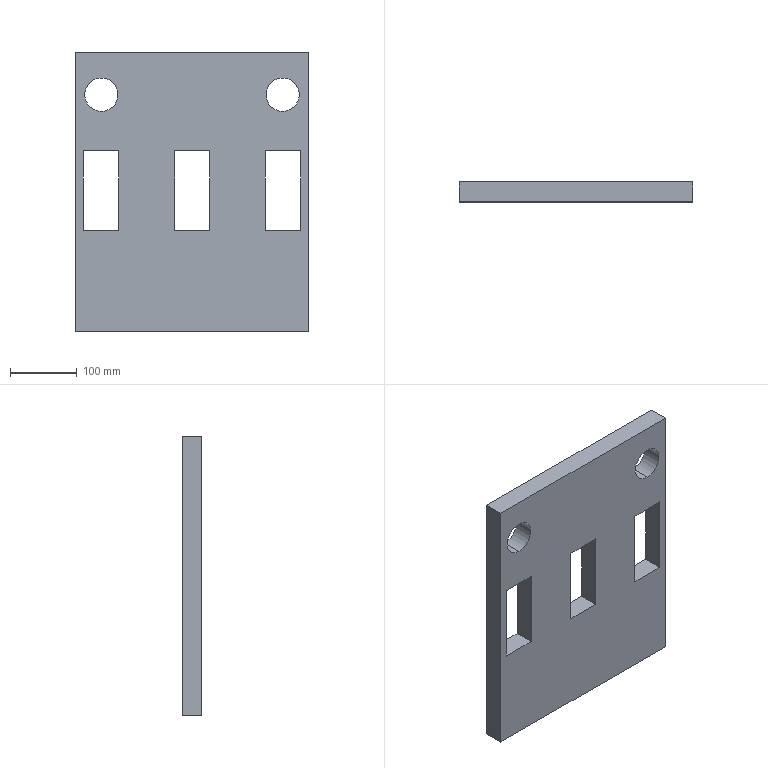Part | SolidWorks | features Extrusion 1 | 1 solid | 22 faces | box 350 x 30 x 420 mm | volume 3719790 mm3 | plane 18 | cylinder 4 | commonest cylinder face diameters 50 x4
STEP:
#1=CARTESIAN_POINT('',(39.,30.,-89.));
#2=VERTEX_POINT('',#1);
#3=CARTESIAN_POINT('',(39.,30.,-39.));
#4=VERTEX_POINT('',#3);
#5=CARTESIAN_POINT('',(39.,30.,-64.));
#6=DIRECTION('',(0.,1.,0.));
#7=DIRECTION('',(0.,0.,1.));
#8=AXIS2_PLACEMENT_3D('',#5,#6,#7);
#9=CIRCLE('',#8,25.);
#10=EDGE_CURVE('',#2,#4,#9,.T.);
#11=ORIENTED_EDGE('',*,*,#10,.T.);
#12=CARTESIAN_POINT('',(39.,0.,-39.));
#13=VERTEX_POINT('',#12);
#14=CARTESIAN_POINT('',(39.,30.,-39.));
#15=DIRECTION('',(0.,-1.,0.));
#16=VECTOR('',#15,1000.);
#17=LINE('',#14,#16);
#18=EDGE_CURVE('',#4,#13,#17,.T.);
#19=ORIENTED_EDGE('',*,*,#18,.T.);
#20=CARTESIAN_POINT('',(39.,0.,-89.));
#21=VERTEX_POINT('',#20);
#22=CARTESIAN_POINT('',(39.,0.,-64.));
#23=DIRECTION('',(0.,1.,0.));
#24=DIRECTION('',(0.,0.,1.));
#25=AXIS2_PLACEMENT_3D('',#22,#23,#24);
#26=CIRCLE('',#25,25.);
#27=EDGE_CURVE('',#21,#13,#26,.T.);
#28=ORIENTED_EDGE('',*,*,#27,.F.);
#29=CARTESIAN_POINT('',(39.,30.,-89.));
#30=DIRECTION('',(0.,-1.,0.));
#31=VECTOR('',#30,1000.);
#32=LINE('',#29,#31);
#33=EDGE_CURVE('',#2,#21,#32,.T.);
#34=ORIENTED_EDGE('',*,*,#33,.F.);
#35=EDGE_LOOP('',(#11,#19,#28,#34));
#36=FACE_OUTER_BOUND('',#35,.T.);
#37=CARTESIAN_POINT('',(39.,30.,-64.));
#38=DIRECTION('',(0.,-1.,0.));
#39=DIRECTION('',(0.,0.,-1.));
#40=AXIS2_PLACEMENT_3D('',#37,#38,#39);
#41=CYLINDRICAL_SURFACE('',#40,25.);
#42=ADVANCED_FACE('',(#36),#41,.F.);
#43=CARTESIAN_POINT('',(311.,30.,-89.));
#44=VERTEX_POINT('',#43);
#45=CARTESIAN_POINT('',(311.,30.,-39.));
#46=VERTEX_POINT('',#45);
#47=CARTESIAN_POINT('',(311.,30.,-64.));
#48=DIRECTION('',(0.,1.,0.));
#49=DIRECTION('',(0.,0.,1.));
#50=AXIS2_PLACEMENT_3D('',#47,#48,#49);
#51=CIRCLE('',#50,25.);
#52=EDGE_CURVE('',#44,#46,#51,.T.);
#53=ORIENTED_EDGE('',*,*,#52,.T.);
#54=CARTESIAN_POINT('',(311.,0.,-39.));
#55=VERTEX_POINT('',#54);
#56=CARTESIAN_POINT('',(311.,30.,-39.));
#57=DIRECTION('',(0.,-1.,0.));
#58=VECTOR('',#57,1000.);
#59=LINE('',#56,#58);
#60=EDGE_CURVE('',#46,#55,#59,.T.);
#61=ORIENTED_EDGE('',*,*,#60,.T.);
#62=CARTESIAN_POINT('',(311.,0.,-89.));
#63=VERTEX_POINT('',#62);
#64=CARTESIAN_POINT('',(311.,0.,-64.));
#65=DIRECTION('',(0.,1.,0.));
#66=DIRECTION('',(0.,0.,1.));
#67=AXIS2_PLACEMENT_3D('',#64,#65,#66);
#68=CIRCLE('',#67,25.);
#69=EDGE_CURVE('',#63,#55,#68,.T.);
#70=ORIENTED_EDGE('',*,*,#69,.F.);
#71=CARTESIAN_POINT('',(311.,30.,-89.));
#72=DIRECTION('',(0.,-1.,0.));
#73=VECTOR('',#72,1000.);
#74=LINE('',#71,#73);
#75=EDGE_CURVE('',#44,#63,#74,.T.);
#76=ORIENTED_EDGE('',*,*,#75,.F.);
#77=EDGE_LOOP('',(#53,#61,#70,#76));
#78=FACE_OUTER_BOUND('',#77,.T.);
#79=CARTESIAN_POINT('',(311.,30.,-64.));
#80=DIRECTION('',(0.,-1.,0.));
#81=DIRECTION('',(0.,0.,-1.));
#82=AXIS2_PLACEMENT_3D('',#79,#80,#81);
#83=CYLINDRICAL_SURFACE('',#82,25.);
#84=ADVANCED_FACE('',(#78),#83,.F.);
#85=ORIENTED_EDGE('',*,*,#52,.F.);
#86=CARTESIAN_POINT('',(311.,30.,-64.));
#87=DIRECTION('',(0.,1.,0.));
#88=DIRECTION('',(0.,0.,1.));
#89=AXIS2_PLACEMENT_3D('',#86,#87,#88);
#90=CIRCLE('',#89,25.);
#91=EDGE_CURVE('',#46,#44,#90,.T.);
#92=ORIENTED_EDGE('',*,*,#91,.F.);
#93=EDGE_LOOP('',(#85,#92));
#94=FACE_BOUND('',#93,.T.);
#95=CARTESIAN_POINT('',(149.,30.,-268.));
#96=VERTEX_POINT('',#95);
#97=CARTESIAN_POINT('',(149.,30.,-148.));
#98=VERTEX_POINT('',#97);
#99=CARTESIAN_POINT('',(149.,30.,-148.));
#100=DIRECTION('',(0.,0.,1.));
#101=VECTOR('',#100,1000.);
#102=LINE('',#99,#101);
#103=EDGE_CURVE('',#96,#98,#102,.T.);
#104=ORIENTED_EDGE('',*,*,#103,.F.);
#105=CARTESIAN_POINT('',(202.,30.,-268.));
#106=VERTEX_POINT('',#105);
#107=CARTESIAN_POINT('',(149.,30.,-268.));
#108=DIRECTION('',(-1.,0.,0.));
#109=VECTOR('',#108,1000.);
#110=LINE('',#107,#109);
#111=EDGE_CURVE('',#106,#96,#110,.T.);
#112=ORIENTED_EDGE('',*,*,#111,.F.);
#113=CARTESIAN_POINT('',(202.,30.,-148.));
#114=VERTEX_POINT('',#113);
#115=CARTESIAN_POINT('',(202.,30.,-268.));
#116=DIRECTION('',(0.,0.,-1.));
#117=VECTOR('',#116,1000.);
#118=LINE('',#115,#117);
#119=EDGE_CURVE('',#114,#106,#118,.T.);
#120=ORIENTED_EDGE('',*,*,#119,.F.);
#121=CARTESIAN_POINT('',(149.,30.,-148.));
#122=DIRECTION('',(1.,0.,0.));
#123=VECTOR('',#122,1000.);
#124=LINE('',#121,#123);
#125=EDGE_CURVE('',#98,#114,#124,.T.);
#126=ORIENTED_EDGE('',*,*,#125,.F.);
#127=EDGE_LOOP('',(#104,#112,#120,#126));
#128=FACE_BOUND('',#127,.T.);
#129=CARTESIAN_POINT('',(0.,30.,-420.));
#130=VERTEX_POINT('',#129);
#131=CARTESIAN_POINT('',(0.,30.,0.));
#132=VERTEX_POINT('',#131);
#133=CARTESIAN_POINT('',(0.,30.,0.));
#134=DIRECTION('',(0.,0.,1.));
#135=VECTOR('',#134,1000.);
#136=LINE('',#133,#135);
#137=EDGE_CURVE('',#130,#132,#136,.T.);
#138=ORIENTED_EDGE('',*,*,#137,.T.);
#139=CARTESIAN_POINT('',(350.,30.,0.));
#140=VERTEX_POINT('',#139);
#141=CARTESIAN_POINT('',(0.,30.,0.));
#142=DIRECTION('',(1.,0.,0.));
#143=VECTOR('',#142,1000.);
#144=LINE('',#141,#143);
#145=EDGE_CURVE('',#132,#140,#144,.T.);
#146=ORIENTED_EDGE('',*,*,#145,.T.);
#147=CARTESIAN_POINT('',(350.,30.,-420.));
#148=VERTEX_POINT('',#147);
#149=CARTESIAN_POINT('',(350.,30.,0.));
#150=DIRECTION('',(0.,0.,-1.));
#151=VECTOR('',#150,1000.);
#152=LINE('',#149,#151);
#153=EDGE_CURVE('',#140,#148,#152,.T.);
#154=ORIENTED_EDGE('',*,*,#153,.T.);
#155=CARTESIAN_POINT('',(0.,30.,-420.));
#156=DIRECTION('',(-1.,0.,0.));
#157=VECTOR('',#156,1000.);
#158=LINE('',#155,#157);
#159=EDGE_CURVE('',#148,#130,#158,.T.);
#160=ORIENTED_EDGE('',*,*,#159,.T.);
#161=EDGE_LOOP('',(#138,#146,#154,#160));
#162=FACE_OUTER_BOUND('',#161,.T.);
#163=CARTESIAN_POINT('',(65.,30.,-268.));
#164=VERTEX_POINT('',#163);
#165=CARTESIAN_POINT('',(12.,30.,-268.));
#166=VERTEX_POINT('',#165);
#167=CARTESIAN_POINT('',(65.,30.,-268.));
#168=DIRECTION('',(-1.,0.,0.));
#169=VECTOR('',#168,1000.);
#170=LINE('',#167,#169);
#171=EDGE_CURVE('',#164,#166,#170,.T.);
#172=ORIENTED_EDGE('',*,*,#171,.F.);
#173=CARTESIAN_POINT('',(65.,30.,-148.));
#174=VERTEX_POINT('',#173);
#175=CARTESIAN_POINT('',(65.,30.,-148.));
#176=DIRECTION('',(0.,0.,-1.));
#177=VECTOR('',#176,1000.);
#178=LINE('',#175,#177);
#179=EDGE_CURVE('',#174,#164,#178,.T.);
#180=ORIENTED_EDGE('',*,*,#179,.F.);
#181=CARTESIAN_POINT('',(12.,30.,-148.));
#182=VERTEX_POINT('',#181);
#183=CARTESIAN_POINT('',(65.,30.,-148.));
#184=DIRECTION('',(1.,0.,0.));
#185=VECTOR('',#184,1000.);
#186=LINE('',#183,#185);
#187=EDGE_CURVE('',#182,#174,#186,.T.);
#188=ORIENTED_EDGE('',*,*,#187,.F.);
#189=CARTESIAN_POINT('',(12.,30.,-268.));
#190=DIRECTION('',(0.,0.,1.));
#191=VECTOR('',#190,1000.);
#192=LINE('',#189,#191);
#193=EDGE_CURVE('',#166,#182,#192,.T.);
#194=ORIENTED_EDGE('',*,*,#193,.F.);
#195=EDGE_LOOP('',(#172,#180,#188,#194));
#196=FACE_BOUND('',#195,.T.);
#197=CARTESIAN_POINT('',(285.,30.,-268.));
#198=VERTEX_POINT('',#197);
#199=CARTESIAN_POINT('',(285.,30.,-148.));
#200=VERTEX_POINT('',#199);
#201=CARTESIAN_POINT('',(285.,30.,-148.));
#202=DIRECTION('',(0.,0.,1.));
#203=VECTOR('',#202,1000.);
#204=LINE('',#201,#203);
#205=EDGE_CURVE('',#198,#200,#204,.T.);
#206=ORIENTED_EDGE('',*,*,#205,.F.);
#207=CARTESIAN_POINT('',(338.,30.,-268.));
#208=VERTEX_POINT('',#207);
#209=CARTESIAN_POINT('',(285.,30.,-268.));
#210=DIRECTION('',(-1.,0.,0.));
#211=VECTOR('',#210,1000.);
#212=LINE('',#209,#211);
#213=EDGE_CURVE('',#208,#198,#212,.T.);
#214=ORIENTED_EDGE('',*,*,#213,.F.);
#215=CARTESIAN_POINT('',(338.,30.,-148.));
#216=VERTEX_POINT('',#215);
#217=CARTESIAN_POINT('',(338.,30.,-268.));
#218=DIRECTION('',(0.,0.,-1.));
#219=VECTOR('',#218,1000.);
#220=LINE('',#217,#219);
#221=EDGE_CURVE('',#216,#208,#220,.T.);
#222=ORIENTED_EDGE('',*,*,#221,.F.);
#223=CARTESIAN_POINT('',(285.,30.,-148.));
#224=DIRECTION('',(1.,0.,0.));
#225=VECTOR('',#224,1000.);
#226=LINE('',#223,#225);
#227=EDGE_CURVE('',#200,#216,#226,.T.);
#228=ORIENTED_EDGE('',*,*,#227,.F.);
#229=EDGE_LOOP('',(#206,#214,#222,#228));
#230=FACE_BOUND('',#229,.T.);
#231=ORIENTED_EDGE('',*,*,#10,.F.);
#232=CARTESIAN_POINT('',(39.,30.,-64.));
#233=DIRECTION('',(0.,1.,0.));
#234=DIRECTION('',(0.,0.,1.));
#235=AXIS2_PLACEMENT_3D('',#232,#233,#234);
#236=CIRCLE('',#235,25.);
#237=EDGE_CURVE('',#4,#2,#236,.T.);
#238=ORIENTED_EDGE('',*,*,#237,.F.);
#239=EDGE_LOOP('',(#231,#238));
#240=FACE_BOUND('',#239,.T.);
#241=CARTESIAN_POINT('',(0.,30.,-420.));
#242=DIRECTION('',(0.,-1.,0.));
#243=DIRECTION('',(0.,0.,-1.));
#244=AXIS2_PLACEMENT_3D('',#241,#242,#243);
#245=PLANE('',#244);
#246=ADVANCED_FACE('',(#94,#128,#162,#196,#230,#240),#245,.F.);
#247=ORIENTED_EDGE('',*,*,#69,.T.);
#248=CARTESIAN_POINT('',(311.,0.,-64.));
#249=DIRECTION('',(0.,1.,0.));
#250=DIRECTION('',(0.,0.,1.));
#251=AXIS2_PLACEMENT_3D('',#248,#249,#250);
#252=CIRCLE('',#251,25.);
#253=EDGE_CURVE('',#55,#63,#252,.T.);
#254=ORIENTED_EDGE('',*,*,#253,.T.);
#255=EDGE_LOOP('',(#247,#254));
#256=FACE_BOUND('',#255,.T.);
#257=CARTESIAN_POINT('',(202.,0.,-268.));
#258=VERTEX_POINT('',#257);
#259=CARTESIAN_POINT('',(149.,0.,-268.));
#260=VERTEX_POINT('',#259);
#261=CARTESIAN_POINT('',(149.,0.,-268.));
#262=DIRECTION('',(-1.,0.,0.));
#263=VECTOR('',#262,1000.);
#264=LINE('',#261,#263);
#265=EDGE_CURVE('',#258,#260,#264,.T.);
#266=ORIENTED_EDGE('',*,*,#265,.T.);
#267=CARTESIAN_POINT('',(149.,0.,-148.));
#268=VERTEX_POINT('',#267);
#269=CARTESIAN_POINT('',(149.,0.,-148.));
#270=DIRECTION('',(0.,0.,1.));
#271=VECTOR('',#270,1000.);
#272=LINE('',#269,#271);
#273=EDGE_CURVE('',#260,#268,#272,.T.);
#274=ORIENTED_EDGE('',*,*,#273,.T.);
#275=CARTESIAN_POINT('',(202.,0.,-148.));
#276=VERTEX_POINT('',#275);
#277=CARTESIAN_POINT('',(149.,0.,-148.));
#278=DIRECTION('',(1.,0.,0.));
#279=VECTOR('',#278,1000.);
#280=LINE('',#277,#279);
#281=EDGE_CURVE('',#268,#276,#280,.T.);
#282=ORIENTED_EDGE('',*,*,#281,.T.);
#283=CARTESIAN_POINT('',(202.,0.,-268.));
#284=DIRECTION('',(0.,0.,-1.));
#285=VECTOR('',#284,1000.);
#286=LINE('',#283,#285);
#287=EDGE_CURVE('',#276,#258,#286,.T.);
#288=ORIENTED_EDGE('',*,*,#287,.T.);
#289=EDGE_LOOP('',(#266,#274,#282,#288));
#290=FACE_BOUND('',#289,.T.);
#291=CARTESIAN_POINT('',(0.,0.,-420.));
#292=VERTEX_POINT('',#291);
#293=CARTESIAN_POINT('',(0.,0.,0.));
#294=VERTEX_POINT('',#293);
#295=CARTESIAN_POINT('',(0.,0.,0.));
#296=DIRECTION('',(0.,0.,1.));
#297=VECTOR('',#296,1000.);
#298=LINE('',#295,#297);
#299=EDGE_CURVE('',#292,#294,#298,.T.);
#300=ORIENTED_EDGE('',*,*,#299,.F.);
#301=CARTESIAN_POINT('',(350.,0.,-420.));
#302=VERTEX_POINT('',#301);
#303=CARTESIAN_POINT('',(0.,0.,-420.));
#304=DIRECTION('',(-1.,0.,0.));
#305=VECTOR('',#304,1000.);
#306=LINE('',#303,#305);
#307=EDGE_CURVE('',#302,#292,#306,.T.);
#308=ORIENTED_EDGE('',*,*,#307,.F.);
#309=CARTESIAN_POINT('',(350.,0.,0.));
#310=VERTEX_POINT('',#309);
#311=CARTESIAN_POINT('',(350.,0.,0.));
#312=DIRECTION('',(0.,0.,-1.));
#313=VECTOR('',#312,1000.);
#314=LINE('',#311,#313);
#315=EDGE_CURVE('',#310,#302,#314,.T.);
#316=ORIENTED_EDGE('',*,*,#315,.F.);
#317=CARTESIAN_POINT('',(0.,0.,0.));
#318=DIRECTION('',(1.,0.,0.));
#319=VECTOR('',#318,1000.);
#320=LINE('',#317,#319);
#321=EDGE_CURVE('',#294,#310,#320,.T.);
#322=ORIENTED_EDGE('',*,*,#321,.F.);
#323=EDGE_LOOP('',(#300,#308,#316,#322));
#324=FACE_OUTER_BOUND('',#323,.T.);
#325=CARTESIAN_POINT('',(65.,0.,-148.));
#326=VERTEX_POINT('',#325);
#327=CARTESIAN_POINT('',(65.,0.,-268.));
#328=VERTEX_POINT('',#327);
#329=CARTESIAN_POINT('',(65.,0.,-148.));
#330=DIRECTION('',(0.,0.,-1.));
#331=VECTOR('',#330,1000.);
#332=LINE('',#329,#331);
#333=EDGE_CURVE('',#326,#328,#332,.T.);
#334=ORIENTED_EDGE('',*,*,#333,.T.);
#335=CARTESIAN_POINT('',(12.,0.,-268.));
#336=VERTEX_POINT('',#335);
#337=CARTESIAN_POINT('',(65.,0.,-268.));
#338=DIRECTION('',(-1.,0.,0.));
#339=VECTOR('',#338,1000.);
#340=LINE('',#337,#339);
#341=EDGE_CURVE('',#328,#336,#340,.T.);
#342=ORIENTED_EDGE('',*,*,#341,.T.);
#343=CARTESIAN_POINT('',(12.,0.,-148.));
#344=VERTEX_POINT('',#343);
#345=CARTESIAN_POINT('',(12.,0.,-268.));
#346=DIRECTION('',(0.,0.,1.));
#347=VECTOR('',#346,1000.);
#348=LINE('',#345,#347);
#349=EDGE_CURVE('',#336,#344,#348,.T.);
#350=ORIENTED_EDGE('',*,*,#349,.T.);
#351=CARTESIAN_POINT('',(65.,0.,-148.));
#352=DIRECTION('',(1.,0.,0.));
#353=VECTOR('',#352,1000.);
#354=LINE('',#351,#353);
#355=EDGE_CURVE('',#344,#326,#354,.T.);
#356=ORIENTED_EDGE('',*,*,#355,.T.);
#357=EDGE_LOOP('',(#334,#342,#350,#356));
#358=FACE_BOUND('',#357,.T.);
#359=CARTESIAN_POINT('',(338.,0.,-268.));
#360=VERTEX_POINT('',#359);
#361=CARTESIAN_POINT('',(285.,0.,-268.));
#362=VERTEX_POINT('',#361);
#363=CARTESIAN_POINT('',(285.,0.,-268.));
#364=DIRECTION('',(-1.,0.,0.));
#365=VECTOR('',#364,1000.);
#366=LINE('',#363,#365);
#367=EDGE_CURVE('',#360,#362,#366,.T.);
#368=ORIENTED_EDGE('',*,*,#367,.T.);
#369=CARTESIAN_POINT('',(285.,0.,-148.));
#370=VERTEX_POINT('',#369);
#371=CARTESIAN_POINT('',(285.,0.,-148.));
#372=DIRECTION('',(0.,0.,1.));
#373=VECTOR('',#372,1000.);
#374=LINE('',#371,#373);
#375=EDGE_CURVE('',#362,#370,#374,.T.);
#376=ORIENTED_EDGE('',*,*,#375,.T.);
#377=CARTESIAN_POINT('',(338.,0.,-148.));
#378=VERTEX_POINT('',#377);
#379=CARTESIAN_POINT('',(285.,0.,-148.));
#380=DIRECTION('',(1.,0.,0.));
#381=VECTOR('',#380,1000.);
#382=LINE('',#379,#381);
#383=EDGE_CURVE('',#370,#378,#382,.T.);
#384=ORIENTED_EDGE('',*,*,#383,.T.);
#385=CARTESIAN_POINT('',(338.,0.,-268.));
#386=DIRECTION('',(0.,0.,-1.));
#387=VECTOR('',#386,1000.);
#388=LINE('',#385,#387);
#389=EDGE_CURVE('',#378,#360,#388,.T.);
#390=ORIENTED_EDGE('',*,*,#389,.T.);
#391=EDGE_LOOP('',(#368,#376,#384,#390));
#392=FACE_BOUND('',#391,.T.);
#393=ORIENTED_EDGE('',*,*,#27,.T.);
#394=CARTESIAN_POINT('',(39.,0.,-64.));
#395=DIRECTION('',(0.,1.,0.));
#396=DIRECTION('',(0.,0.,1.));
#397=AXIS2_PLACEMENT_3D('',#394,#395,#396);
#398=CIRCLE('',#397,25.);
#399=EDGE_CURVE('',#13,#21,#398,.T.);
#400=ORIENTED_EDGE('',*,*,#399,.T.);
#401=EDGE_LOOP('',(#393,#400));
#402=FACE_BOUND('',#401,.T.);
#403=CARTESIAN_POINT('',(0.,0.,-420.));
#404=DIRECTION('',(0.,-1.,0.));
#405=DIRECTION('',(0.,0.,-1.));
#406=AXIS2_PLACEMENT_3D('',#403,#404,#405);
#407=PLANE('',#406);
#408=ADVANCED_FACE('',(#256,#290,#324,#358,#392,#402),#407,.T.);
#409=ORIENTED_EDGE('',*,*,#299,.T.);
#410=CARTESIAN_POINT('',(0.,30.,0.));
#411=DIRECTION('',(0.,-1.,0.));
#412=VECTOR('',#411,1000.);
#413=LINE('',#410,#412);
#414=EDGE_CURVE('',#132,#294,#413,.T.);
#415=ORIENTED_EDGE('',*,*,#414,.F.);
#416=ORIENTED_EDGE('',*,*,#137,.F.);
#417=CARTESIAN_POINT('',(0.,30.,-420.));
#418=DIRECTION('',(0.,-1.,0.));
#419=VECTOR('',#418,1000.);
#420=LINE('',#417,#419);
#421=EDGE_CURVE('',#130,#292,#420,.T.);
#422=ORIENTED_EDGE('',*,*,#421,.T.);
#423=EDGE_LOOP('',(#409,#415,#416,#422));
#424=FACE_OUTER_BOUND('',#423,.T.);
#425=CARTESIAN_POINT('',(0.,30.,0.));
#426=DIRECTION('',(1.,0.,0.));
#427=DIRECTION('',(0.,0.,-1.));
#428=AXIS2_PLACEMENT_3D('',#425,#426,#427);
#429=PLANE('',#428);
#430=ADVANCED_FACE('',(#424),#429,.F.);
#431=ORIENTED_EDGE('',*,*,#321,.T.);
#432=CARTESIAN_POINT('',(350.,30.,0.));
#433=DIRECTION('',(0.,-1.,0.));
#434=VECTOR('',#433,1000.);
#435=LINE('',#432,#434);
#436=EDGE_CURVE('',#140,#310,#435,.T.);
#437=ORIENTED_EDGE('',*,*,#436,.F.);
#438=ORIENTED_EDGE('',*,*,#145,.F.);
#439=ORIENTED_EDGE('',*,*,#414,.T.);
#440=EDGE_LOOP('',(#431,#437,#438,#439));
#441=FACE_OUTER_BOUND('',#440,.T.);
#442=CARTESIAN_POINT('',(0.,30.,0.));
#443=DIRECTION('',(0.,0.,-1.));
#444=DIRECTION('',(-1.,0.,0.));
#445=AXIS2_PLACEMENT_3D('',#442,#443,#444);
#446=PLANE('',#445);
#447=ADVANCED_FACE('',(#441),#446,.F.);
#448=ORIENTED_EDGE('',*,*,#315,.T.);
#449=CARTESIAN_POINT('',(350.,30.,-420.));
#450=DIRECTION('',(0.,-1.,0.));
#451=VECTOR('',#450,1000.);
#452=LINE('',#449,#451);
#453=EDGE_CURVE('',#148,#302,#452,.T.);
#454=ORIENTED_EDGE('',*,*,#453,.F.);
#455=ORIENTED_EDGE('',*,*,#153,.F.);
#456=ORIENTED_EDGE('',*,*,#436,.T.);
#457=EDGE_LOOP('',(#448,#454,#455,#456));
#458=FACE_OUTER_BOUND('',#457,.T.);
#459=CARTESIAN_POINT('',(350.,30.,0.));
#460=DIRECTION('',(-1.,0.,0.));
#461=DIRECTION('',(0.,0.,1.));
#462=AXIS2_PLACEMENT_3D('',#459,#460,#461);
#463=PLANE('',#462);
#464=ADVANCED_FACE('',(#458),#463,.F.);
#465=ORIENTED_EDGE('',*,*,#307,.T.);
#466=ORIENTED_EDGE('',*,*,#421,.F.);
#467=ORIENTED_EDGE('',*,*,#159,.F.);
#468=ORIENTED_EDGE('',*,*,#453,.T.);
#469=EDGE_LOOP('',(#465,#466,#467,#468));
#470=FACE_OUTER_BOUND('',#469,.T.);
#471=CARTESIAN_POINT('',(0.,30.,-420.));
#472=DIRECTION('',(0.,0.,1.));
#473=DIRECTION('',(1.,0.,0.));
#474=AXIS2_PLACEMENT_3D('',#471,#472,#473);
#475=PLANE('',#474);
#476=ADVANCED_FACE('',(#470),#475,.F.);
#477=ORIENTED_EDGE('',*,*,#341,.F.);
#478=CARTESIAN_POINT('',(65.,30.,-268.));
#479=DIRECTION('',(0.,-1.,0.));
#480=VECTOR('',#479,1000.);
#481=LINE('',#478,#480);
#482=EDGE_CURVE('',#164,#328,#481,.T.);
#483=ORIENTED_EDGE('',*,*,#482,.F.);
#484=ORIENTED_EDGE('',*,*,#171,.T.);
#485=CARTESIAN_POINT('',(12.,30.,-268.));
#486=DIRECTION('',(0.,-1.,0.));
#487=VECTOR('',#486,1000.);
#488=LINE('',#485,#487);
#489=EDGE_CURVE('',#166,#336,#488,.T.);
#490=ORIENTED_EDGE('',*,*,#489,.T.);
#491=EDGE_LOOP('',(#477,#483,#484,#490));
#492=FACE_OUTER_BOUND('',#491,.T.);
#493=CARTESIAN_POINT('',(65.,30.,-268.));
#494=DIRECTION('',(0.,0.,1.));
#495=DIRECTION('',(1.,0.,0.));
#496=AXIS2_PLACEMENT_3D('',#493,#494,#495);
#497=PLANE('',#496);
#498=ADVANCED_FACE('',(#492),#497,.T.);
#499=ORIENTED_EDGE('',*,*,#349,.F.);
#500=ORIENTED_EDGE('',*,*,#489,.F.);
#501=ORIENTED_EDGE('',*,*,#193,.T.);
#502=CARTESIAN_POINT('',(12.,30.,-148.));
#503=DIRECTION('',(0.,-1.,0.));
#504=VECTOR('',#503,1000.);
#505=LINE('',#502,#504);
#506=EDGE_CURVE('',#182,#344,#505,.T.);
#507=ORIENTED_EDGE('',*,*,#506,.T.);
#508=EDGE_LOOP('',(#499,#500,#501,#507));
#509=FACE_OUTER_BOUND('',#508,.T.);
#510=CARTESIAN_POINT('',(12.,30.,-268.));
#511=DIRECTION('',(1.,0.,0.));
#512=DIRECTION('',(0.,0.,-1.));
#513=AXIS2_PLACEMENT_3D('',#510,#511,#512);
#514=PLANE('',#513);
#515=ADVANCED_FACE('',(#509),#514,.T.);
#516=ORIENTED_EDGE('',*,*,#355,.F.);
#517=ORIENTED_EDGE('',*,*,#506,.F.);
#518=ORIENTED_EDGE('',*,*,#187,.T.);
#519=CARTESIAN_POINT('',(65.,30.,-148.));
#520=DIRECTION('',(0.,-1.,0.));
#521=VECTOR('',#520,1000.);
#522=LINE('',#519,#521);
#523=EDGE_CURVE('',#174,#326,#522,.T.);
#524=ORIENTED_EDGE('',*,*,#523,.T.);
#525=EDGE_LOOP('',(#516,#517,#518,#524));
#526=FACE_OUTER_BOUND('',#525,.T.);
#527=CARTESIAN_POINT('',(65.,30.,-148.));
#528=DIRECTION('',(0.,0.,-1.));
#529=DIRECTION('',(-1.,0.,0.));
#530=AXIS2_PLACEMENT_3D('',#527,#528,#529);
#531=PLANE('',#530);
#532=ADVANCED_FACE('',(#526),#531,.T.);
#533=ORIENTED_EDGE('',*,*,#333,.F.);
#534=ORIENTED_EDGE('',*,*,#523,.F.);
#535=ORIENTED_EDGE('',*,*,#179,.T.);
#536=ORIENTED_EDGE('',*,*,#482,.T.);
#537=EDGE_LOOP('',(#533,#534,#535,#536));
#538=FACE_OUTER_BOUND('',#537,.T.);
#539=CARTESIAN_POINT('',(65.,30.,-148.));
#540=DIRECTION('',(-1.,0.,0.));
#541=DIRECTION('',(0.,0.,1.));
#542=AXIS2_PLACEMENT_3D('',#539,#540,#541);
#543=PLANE('',#542);
#544=ADVANCED_FACE('',(#538),#543,.T.);
#545=ORIENTED_EDGE('',*,*,#273,.F.);
#546=CARTESIAN_POINT('',(149.,30.,-268.));
#547=DIRECTION('',(0.,-1.,0.));
#548=VECTOR('',#547,1000.);
#549=LINE('',#546,#548);
#550=EDGE_CURVE('',#96,#260,#549,.T.);
#551=ORIENTED_EDGE('',*,*,#550,.F.);
#552=ORIENTED_EDGE('',*,*,#103,.T.);
#553=CARTESIAN_POINT('',(149.,30.,-148.));
#554=DIRECTION('',(0.,-1.,0.));
#555=VECTOR('',#554,1000.);
#556=LINE('',#553,#555);
#557=EDGE_CURVE('',#98,#268,#556,.T.);
#558=ORIENTED_EDGE('',*,*,#557,.T.);
#559=EDGE_LOOP('',(#545,#551,#552,#558));
#560=FACE_OUTER_BOUND('',#559,.T.);
#561=CARTESIAN_POINT('',(149.,30.,-148.));
#562=DIRECTION('',(1.,0.,0.));
#563=DIRECTION('',(0.,0.,-1.));
#564=AXIS2_PLACEMENT_3D('',#561,#562,#563);
#565=PLANE('',#564);
#566=ADVANCED_FACE('',(#560),#565,.T.);
#567=ORIENTED_EDGE('',*,*,#281,.F.);
#568=ORIENTED_EDGE('',*,*,#557,.F.);
#569=ORIENTED_EDGE('',*,*,#125,.T.);
#570=CARTESIAN_POINT('',(202.,30.,-148.));
#571=DIRECTION('',(0.,-1.,0.));
#572=VECTOR('',#571,1000.);
#573=LINE('',#570,#572);
#574=EDGE_CURVE('',#114,#276,#573,.T.);
#575=ORIENTED_EDGE('',*,*,#574,.T.);
#576=EDGE_LOOP('',(#567,#568,#569,#575));
#577=FACE_OUTER_BOUND('',#576,.T.);
#578=CARTESIAN_POINT('',(149.,30.,-148.));
#579=DIRECTION('',(0.,0.,-1.));
#580=DIRECTION('',(-1.,0.,0.));
#581=AXIS2_PLACEMENT_3D('',#578,#579,#580);
#582=PLANE('',#581);
#583=ADVANCED_FACE('',(#577),#582,.T.);
#584=ORIENTED_EDGE('',*,*,#287,.F.);
#585=ORIENTED_EDGE('',*,*,#574,.F.);
#586=ORIENTED_EDGE('',*,*,#119,.T.);
#587=CARTESIAN_POINT('',(202.,30.,-268.));
#588=DIRECTION('',(0.,-1.,0.));
#589=VECTOR('',#588,1000.);
#590=LINE('',#587,#589);
#591=EDGE_CURVE('',#106,#258,#590,.T.);
#592=ORIENTED_EDGE('',*,*,#591,.T.);
#593=EDGE_LOOP('',(#584,#585,#586,#592));
#594=FACE_OUTER_BOUND('',#593,.T.);
#595=CARTESIAN_POINT('',(202.,30.,-268.));
#596=DIRECTION('',(-1.,0.,0.));
#597=DIRECTION('',(0.,0.,1.));
#598=AXIS2_PLACEMENT_3D('',#595,#596,#597);
#599=PLANE('',#598);
#600=ADVANCED_FACE('',(#594),#599,.T.);
#601=ORIENTED_EDGE('',*,*,#265,.F.);
#602=ORIENTED_EDGE('',*,*,#591,.F.);
#603=ORIENTED_EDGE('',*,*,#111,.T.);
#604=ORIENTED_EDGE('',*,*,#550,.T.);
#605=EDGE_LOOP('',(#601,#602,#603,#604));
#606=FACE_OUTER_BOUND('',#605,.T.);
#607=CARTESIAN_POINT('',(149.,30.,-268.));
#608=DIRECTION('',(0.,0.,1.));
#609=DIRECTION('',(1.,0.,0.));
#610=AXIS2_PLACEMENT_3D('',#607,#608,#609);
#611=PLANE('',#610);
#612=ADVANCED_FACE('',(#606),#611,.T.);
#613=ORIENTED_EDGE('',*,*,#375,.F.);
#614=CARTESIAN_POINT('',(285.,30.,-268.));
#615=DIRECTION('',(0.,-1.,0.));
#616=VECTOR('',#615,1000.);
#617=LINE('',#614,#616);
#618=EDGE_CURVE('',#198,#362,#617,.T.);
#619=ORIENTED_EDGE('',*,*,#618,.F.);
#620=ORIENTED_EDGE('',*,*,#205,.T.);
#621=CARTESIAN_POINT('',(285.,30.,-148.));
#622=DIRECTION('',(0.,-1.,0.));
#623=VECTOR('',#622,1000.);
#624=LINE('',#621,#623);
#625=EDGE_CURVE('',#200,#370,#624,.T.);
#626=ORIENTED_EDGE('',*,*,#625,.T.);
#627=EDGE_LOOP('',(#613,#619,#620,#626));
#628=FACE_OUTER_BOUND('',#627,.T.);
#629=CARTESIAN_POINT('',(285.,30.,-148.));
#630=DIRECTION('',(1.,0.,0.));
#631=DIRECTION('',(0.,0.,-1.));
#632=AXIS2_PLACEMENT_3D('',#629,#630,#631);
#633=PLANE('',#632);
#634=ADVANCED_FACE('',(#628),#633,.T.);
#635=ORIENTED_EDGE('',*,*,#383,.F.);
#636=ORIENTED_EDGE('',*,*,#625,.F.);
#637=ORIENTED_EDGE('',*,*,#227,.T.);
#638=CARTESIAN_POINT('',(338.,30.,-148.));
#639=DIRECTION('',(0.,-1.,0.));
#640=VECTOR('',#639,1000.);
#641=LINE('',#638,#640);
#642=EDGE_CURVE('',#216,#378,#641,.T.);
#643=ORIENTED_EDGE('',*,*,#642,.T.);
#644=EDGE_LOOP('',(#635,#636,#637,#643));
#645=FACE_OUTER_BOUND('',#644,.T.);
#646=CARTESIAN_POINT('',(285.,30.,-148.));
#647=DIRECTION('',(0.,0.,-1.));
#648=DIRECTION('',(-1.,0.,0.));
#649=AXIS2_PLACEMENT_3D('',#646,#647,#648);
#650=PLANE('',#649);
#651=ADVANCED_FACE('',(#645),#650,.T.);
#652=ORIENTED_EDGE('',*,*,#389,.F.);
#653=ORIENTED_EDGE('',*,*,#642,.F.);
#654=ORIENTED_EDGE('',*,*,#221,.T.);
#655=CARTESIAN_POINT('',(338.,30.,-268.));
#656=DIRECTION('',(0.,-1.,0.));
#657=VECTOR('',#656,1000.);
#658=LINE('',#655,#657);
#659=EDGE_CURVE('',#208,#360,#658,.T.);
#660=ORIENTED_EDGE('',*,*,#659,.T.);
#661=EDGE_LOOP('',(#652,#653,#654,#660));
#662=FACE_OUTER_BOUND('',#661,.T.);
#663=CARTESIAN_POINT('',(338.,30.,-268.));
#664=DIRECTION('',(-1.,0.,0.));
#665=DIRECTION('',(0.,0.,1.));
#666=AXIS2_PLACEMENT_3D('',#663,#664,#665);
#667=PLANE('',#666);
#668=ADVANCED_FACE('',(#662),#667,.T.);
#669=ORIENTED_EDGE('',*,*,#367,.F.);
#670=ORIENTED_EDGE('',*,*,#659,.F.);
#671=ORIENTED_EDGE('',*,*,#213,.T.);
#672=ORIENTED_EDGE('',*,*,#618,.T.);
#673=EDGE_LOOP('',(#669,#670,#671,#672));
#674=FACE_OUTER_BOUND('',#673,.T.);
#675=CARTESIAN_POINT('',(285.,30.,-268.));
#676=DIRECTION('',(0.,0.,1.));
#677=DIRECTION('',(1.,0.,0.));
#678=AXIS2_PLACEMENT_3D('',#675,#676,#677);
#679=PLANE('',#678);
#680=ADVANCED_FACE('',(#674),#679,.T.);
#681=ORIENTED_EDGE('',*,*,#60,.F.);
#682=ORIENTED_EDGE('',*,*,#91,.T.);
#683=ORIENTED_EDGE('',*,*,#75,.T.);
#684=ORIENTED_EDGE('',*,*,#253,.F.);
#685=EDGE_LOOP('',(#681,#682,#683,#684));
#686=FACE_OUTER_BOUND('',#685,.T.);
#687=CARTESIAN_POINT('',(311.,30.,-64.));
#688=DIRECTION('',(0.,-1.,0.));
#689=DIRECTION('',(0.,0.,-1.));
#690=AXIS2_PLACEMENT_3D('',#687,#688,#689);
#691=CYLINDRICAL_SURFACE('',#690,25.);
#692=ADVANCED_FACE('',(#686),#691,.F.);
#693=ORIENTED_EDGE('',*,*,#18,.F.);
#694=ORIENTED_EDGE('',*,*,#237,.T.);
#695=ORIENTED_EDGE('',*,*,#33,.T.);
#696=ORIENTED_EDGE('',*,*,#399,.F.);
#697=EDGE_LOOP('',(#693,#694,#695,#696));
#698=FACE_OUTER_BOUND('',#697,.T.);
#699=CARTESIAN_POINT('',(39.,30.,-64.));
#700=DIRECTION('',(0.,-1.,0.));
#701=DIRECTION('',(0.,0.,-1.));
#702=AXIS2_PLACEMENT_3D('',#699,#700,#701);
#703=CYLINDRICAL_SURFACE('',#702,25.);
#704=ADVANCED_FACE('',(#698),#703,.F.);
#705=CLOSED_SHELL('',(#42,#84,#246,#408,#430,#447,#464,#476,#498,#515,#532,#544,#566,#583,#600,#612,#634,#651,#668,#680,#692,#704));
#706=MANIFOLD_SOLID_BREP('',#705);
#707=CARTESIAN_POINT('',(0.,0.,0.));
#708=DIRECTION('',(0.,0.,1.));
#709=DIRECTION('',(1.,0.,0.));
#710=AXIS2_PLACEMENT_3D('',#707,#708,#709);
#711=(LENGTH_UNIT()NAMED_UNIT(*)SI_UNIT(.MILLI.,.METRE.));
#712=UNCERTAINTY_MEASURE_WITH_UNIT(LENGTH_MEASURE(0.00001),#711,'','');
#713=(NAMED_UNIT(*)PLANE_ANGLE_UNIT()SI_UNIT($,.RADIAN.));
#714=(NAMED_UNIT(*)SI_UNIT($,.STERADIAN.)SOLID_ANGLE_UNIT());
#715=(GEOMETRIC_REPRESENTATION_CONTEXT(3)GLOBAL_UNCERTAINTY_ASSIGNED_CONTEXT((#712))GLOBAL_UNIT_ASSIGNED_CONTEXT((#711,#713,#714))REPRESENTATION_CONTEXT('',''));
#716=ADVANCED_BREP_SHAPE_REPRESENTATION('',(#706,#710),#715);